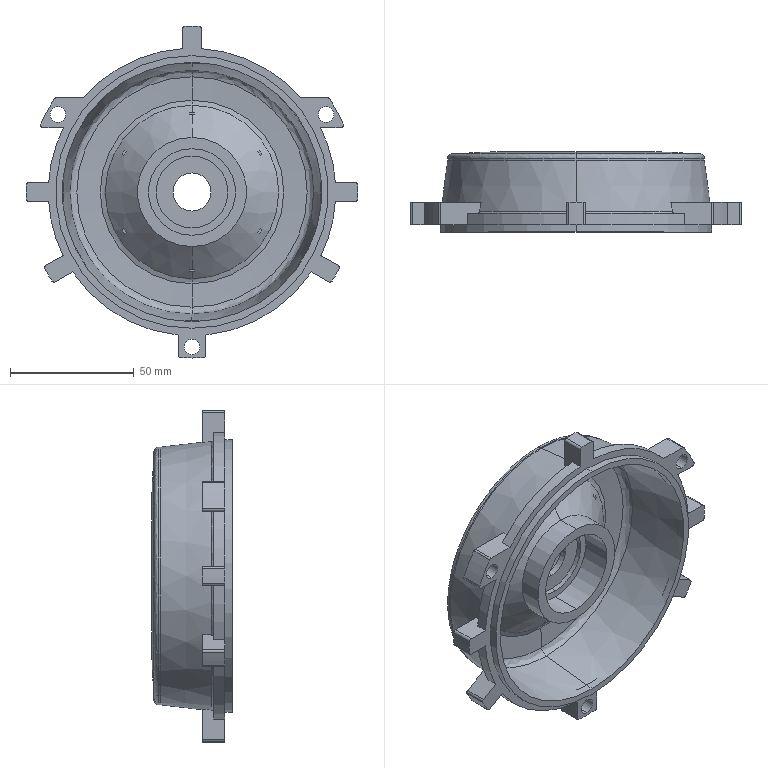Part | SolidWorks | features BaseBody 1 | 1 solid | 202 faces | box 134 x 32.5 x 134 mm | volume 79781 mm3 | plane 89 | cylinder 75 | spline 22 | cone 16 | commonest cylinder face diameters 2 x18 104 x11 64 x9 134 x9 116 x8 6.3 x6